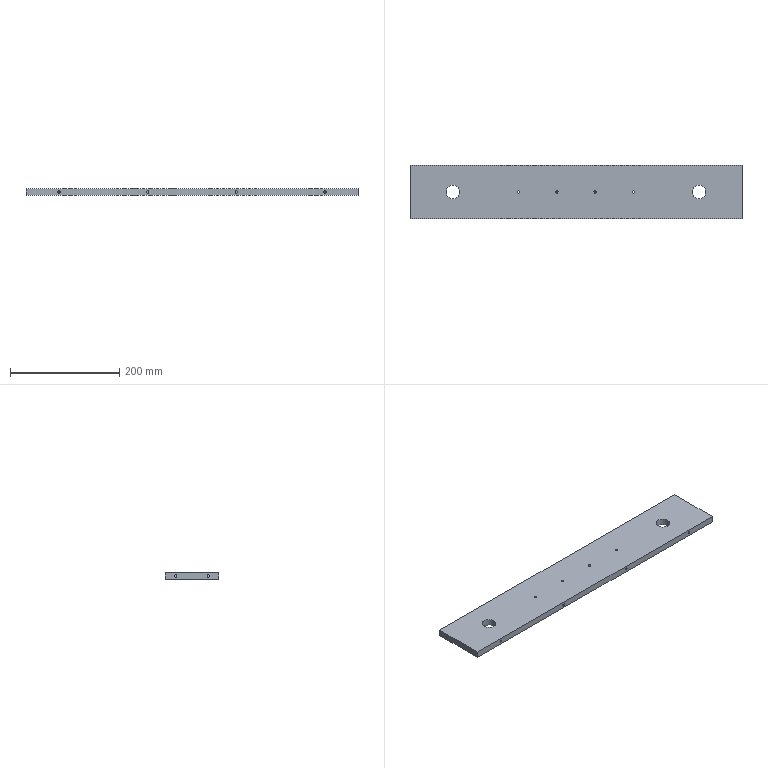Part | STEP file | Shim mounting plate base | 1 solid | 54 faces | box 607 x 98 x 12 mm | volume 699324 mm3 | cylinder 36 | plane 18 | commonest cylinder face diameters 4.2 x32 25 x4